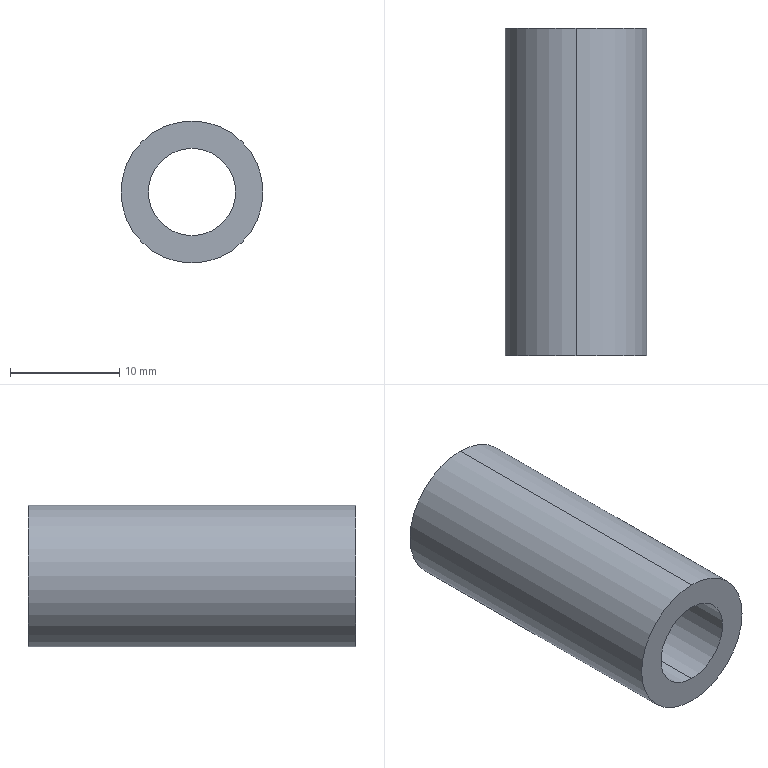Part | STEP file | Ball joint spacer | 1 solid | 6 faces | box 13 x 30 x 13 mm | volume 2474 mm3 | cylinder 4 | plane 2 | commonest cylinder face diameters 8 x2 13 x2
STEP:
#1=CARTESIAN_POINT('',(0.,0.,0.));
#2=DIRECTION('',(0.,0.,1.));
#3=DIRECTION('',(1.,0.,0.));
#4=AXIS2_PLACEMENT_3D('',#1,#2,#3);
#5=CARTESIAN_POINT('',(0.,30.,-4.));
#6=VERTEX_POINT('',#5);
#7=CARTESIAN_POINT('',(0.,0.,-4.));
#8=VERTEX_POINT('',#7);
#9=CARTESIAN_POINT('',(0.,30.,-4.));
#10=DIRECTION('',(0.,-1.,0.));
#11=VECTOR('',#10,1.);
#12=LINE('',#9,#11);
#13=CARTESIAN_POINT('',(0.,30.,0.));
#14=DIRECTION('',(0.,-1.,0.));
#15=DIRECTION('',(0.,0.,-1.));
#16=AXIS2_PLACEMENT_3D('',#13,#14,#15);
#17=CYLINDRICAL_SURFACE('',#16,4.);
#18=CARTESIAN_POINT('',(6.283,0.));
#19=DIRECTION('',(0.,1.));
#20=VECTOR('',#19,1.);
#21=LINE('',#18,#20);
#22=(GEOMETRIC_REPRESENTATION_CONTEXT(2)PARAMETRIC_REPRESENTATION_CONTEXT()REPRESENTATION_CONTEXT('',''));
#23=DEFINITIONAL_REPRESENTATION('',(#21),#22);
#24=PCURVE('',#17,#23);
#25=CARTESIAN_POINT('',(0.,30.,0.));
#26=DIRECTION('',(0.,-1.,0.));
#27=DIRECTION('',(0.,0.,-1.));
#28=AXIS2_PLACEMENT_3D('',#25,#26,#27);
#29=CYLINDRICAL_SURFACE('',#28,4.);
#30=CARTESIAN_POINT('',(0.,0.));
#31=DIRECTION('',(0.,1.));
#32=VECTOR('',#31,1.);
#33=LINE('',#30,#32);
#34=(GEOMETRIC_REPRESENTATION_CONTEXT(2)PARAMETRIC_REPRESENTATION_CONTEXT()REPRESENTATION_CONTEXT('',''));
#35=DEFINITIONAL_REPRESENTATION('',(#33),#34);
#36=PCURVE('',#29,#35);
#37=SURFACE_CURVE('',#12,(#24,#36),.PCURVE_S1.);
#38=EDGE_CURVE('',#6,#8,#37,.T.);
#39=ORIENTED_EDGE('',*,*,#38,.T.);
#40=CARTESIAN_POINT('',(0.,0.,4.));
#41=VERTEX_POINT('',#40);
#42=CARTESIAN_POINT('',(0.,0.,0.));
#43=DIRECTION('',(0.,1.,0.));
#44=DIRECTION('',(0.,0.,1.));
#45=AXIS2_PLACEMENT_3D('',#42,#43,#44);
#46=CIRCLE('',#45,4.);
#47=CARTESIAN_POINT('',(9.425,30.));
#48=DIRECTION('',(-1.,0.));
#49=VECTOR('',#48,1.);
#50=LINE('',#47,#49);
#51=(GEOMETRIC_REPRESENTATION_CONTEXT(2)PARAMETRIC_REPRESENTATION_CONTEXT()REPRESENTATION_CONTEXT('',''));
#52=DEFINITIONAL_REPRESENTATION('',(#50),#51);
#53=PCURVE('',#17,#52);
#54=CARTESIAN_POINT('',(0.,0.,0.));
#55=DIRECTION('',(0.,1.,0.));
#56=DIRECTION('',(0.,0.,1.));
#57=AXIS2_PLACEMENT_3D('',#54,#55,#56);
#58=PLANE('',#57);
#59=CARTESIAN_POINT('',(0.,0.));
#60=DIRECTION('',(1.,0.));
#61=AXIS2_PLACEMENT_2D('',#59,#60);
#62=CIRCLE('',#61,4.);
#63=(GEOMETRIC_REPRESENTATION_CONTEXT(2)PARAMETRIC_REPRESENTATION_CONTEXT()REPRESENTATION_CONTEXT('',''));
#64=DEFINITIONAL_REPRESENTATION('',(#62),#63);
#65=PCURVE('',#58,#64);
#66=SURFACE_CURVE('',#46,(#53,#65),.PCURVE_S1.);
#67=EDGE_CURVE('',#8,#41,#66,.T.);
#68=ORIENTED_EDGE('',*,*,#67,.T.);
#69=CARTESIAN_POINT('',(0.,30.,4.));
#70=VERTEX_POINT('',#69);
#71=CARTESIAN_POINT('',(0.,30.,4.));
#72=DIRECTION('',(0.,-1.,0.));
#73=VECTOR('',#72,1.);
#74=LINE('',#71,#73);
#75=CARTESIAN_POINT('',(3.142,0.));
#76=DIRECTION('',(0.,1.));
#77=VECTOR('',#76,1.);
#78=LINE('',#75,#77);
#79=(GEOMETRIC_REPRESENTATION_CONTEXT(2)PARAMETRIC_REPRESENTATION_CONTEXT()REPRESENTATION_CONTEXT('',''));
#80=DEFINITIONAL_REPRESENTATION('',(#78),#79);
#81=PCURVE('',#17,#80);
#82=CARTESIAN_POINT('',(3.142,0.));
#83=DIRECTION('',(0.,1.));
#84=VECTOR('',#83,1.);
#85=LINE('',#82,#84);
#86=(GEOMETRIC_REPRESENTATION_CONTEXT(2)PARAMETRIC_REPRESENTATION_CONTEXT()REPRESENTATION_CONTEXT('',''));
#87=DEFINITIONAL_REPRESENTATION('',(#85),#86);
#88=PCURVE('',#29,#87);
#89=SURFACE_CURVE('',#74,(#81,#88),.PCURVE_S1.);
#90=EDGE_CURVE('',#70,#41,#89,.T.);
#91=ORIENTED_EDGE('',*,*,#90,.F.);
#92=CARTESIAN_POINT('',(0.,30.,0.));
#93=DIRECTION('',(0.,1.,0.));
#94=DIRECTION('',(0.,0.,1.));
#95=AXIS2_PLACEMENT_3D('',#92,#93,#94);
#96=CIRCLE('',#95,4.);
#97=CARTESIAN_POINT('',(9.425,0.));
#98=DIRECTION('',(-1.,0.));
#99=VECTOR('',#98,1.);
#100=LINE('',#97,#99);
#101=(GEOMETRIC_REPRESENTATION_CONTEXT(2)PARAMETRIC_REPRESENTATION_CONTEXT()REPRESENTATION_CONTEXT('',''));
#102=DEFINITIONAL_REPRESENTATION('',(#100),#101);
#103=PCURVE('',#17,#102);
#104=CARTESIAN_POINT('',(0.,30.,0.));
#105=DIRECTION('',(0.,1.,0.));
#106=DIRECTION('',(0.,0.,1.));
#107=AXIS2_PLACEMENT_3D('',#104,#105,#106);
#108=PLANE('',#107);
#109=CARTESIAN_POINT('',(0.,0.));
#110=DIRECTION('',(1.,0.));
#111=AXIS2_PLACEMENT_2D('',#109,#110);
#112=CIRCLE('',#111,4.);
#113=(GEOMETRIC_REPRESENTATION_CONTEXT(2)PARAMETRIC_REPRESENTATION_CONTEXT()REPRESENTATION_CONTEXT('',''));
#114=DEFINITIONAL_REPRESENTATION('',(#112),#113);
#115=PCURVE('',#108,#114);
#116=SURFACE_CURVE('',#96,(#103,#115),.PCURVE_S1.);
#117=EDGE_CURVE('',#6,#70,#116,.T.);
#118=ORIENTED_EDGE('',*,*,#117,.F.);
#119=EDGE_LOOP('',(#39,#68,#91,#118));
#120=FACE_BOUND('',#119,.F.);
#121=ADVANCED_FACE('',(#120),#17,.F.);
#122=CARTESIAN_POINT('',(0.,30.,6.5));
#123=VERTEX_POINT('',#122);
#124=CARTESIAN_POINT('',(0.,30.,-6.5));
#125=VERTEX_POINT('',#124);
#126=CARTESIAN_POINT('',(0.,30.,0.));
#127=DIRECTION('',(0.,1.,0.));
#128=DIRECTION('',(0.,0.,1.));
#129=AXIS2_PLACEMENT_3D('',#126,#127,#128);
#130=CIRCLE('',#129,6.5);
#131=CARTESIAN_POINT('',(0.,30.,0.));
#132=DIRECTION('',(0.,-1.,0.));
#133=DIRECTION('',(0.,0.,-1.));
#134=AXIS2_PLACEMENT_3D('',#131,#132,#133);
#135=CYLINDRICAL_SURFACE('',#134,6.5);
#136=CARTESIAN_POINT('',(3.142,0.));
#137=DIRECTION('',(-1.,0.));
#138=VECTOR('',#137,1.);
#139=LINE('',#136,#138);
#140=(GEOMETRIC_REPRESENTATION_CONTEXT(2)PARAMETRIC_REPRESENTATION_CONTEXT()REPRESENTATION_CONTEXT('',''));
#141=DEFINITIONAL_REPRESENTATION('',(#139),#140);
#142=PCURVE('',#135,#141);
#143=CARTESIAN_POINT('',(0.,0.));
#144=DIRECTION('',(1.,0.));
#145=AXIS2_PLACEMENT_2D('',#143,#144);
#146=CIRCLE('',#145,6.5);
#147=(GEOMETRIC_REPRESENTATION_CONTEXT(2)PARAMETRIC_REPRESENTATION_CONTEXT()REPRESENTATION_CONTEXT('',''));
#148=DEFINITIONAL_REPRESENTATION('',(#146),#147);
#149=PCURVE('',#108,#148);
#150=SURFACE_CURVE('',#130,(#142,#149),.PCURVE_S1.);
#151=EDGE_CURVE('',#123,#125,#150,.T.);
#152=ORIENTED_EDGE('',*,*,#151,.F.);
#153=CARTESIAN_POINT('',(0.,0.,6.5));
#154=VERTEX_POINT('',#153);
#155=CARTESIAN_POINT('',(0.,30.,6.5));
#156=DIRECTION('',(0.,-1.,0.));
#157=VECTOR('',#156,1.);
#158=LINE('',#155,#157);
#159=CARTESIAN_POINT('',(3.142,0.));
#160=DIRECTION('',(0.,1.));
#161=VECTOR('',#160,1.);
#162=LINE('',#159,#161);
#163=(GEOMETRIC_REPRESENTATION_CONTEXT(2)PARAMETRIC_REPRESENTATION_CONTEXT()REPRESENTATION_CONTEXT('',''));
#164=DEFINITIONAL_REPRESENTATION('',(#162),#163);
#165=PCURVE('',#135,#164);
#166=CARTESIAN_POINT('',(0.,30.,0.));
#167=DIRECTION('',(0.,-1.,0.));
#168=DIRECTION('',(0.,0.,-1.));
#169=AXIS2_PLACEMENT_3D('',#166,#167,#168);
#170=CYLINDRICAL_SURFACE('',#169,6.5);
#171=CARTESIAN_POINT('',(3.142,0.));
#172=DIRECTION('',(0.,1.));
#173=VECTOR('',#172,1.);
#174=LINE('',#171,#173);
#175=(GEOMETRIC_REPRESENTATION_CONTEXT(2)PARAMETRIC_REPRESENTATION_CONTEXT()REPRESENTATION_CONTEXT('',''));
#176=DEFINITIONAL_REPRESENTATION('',(#174),#175);
#177=PCURVE('',#170,#176);
#178=SURFACE_CURVE('',#158,(#165,#177),.PCURVE_S1.);
#179=EDGE_CURVE('',#123,#154,#178,.T.);
#180=ORIENTED_EDGE('',*,*,#179,.T.);
#181=CARTESIAN_POINT('',(0.,0.,-6.5));
#182=VERTEX_POINT('',#181);
#183=CARTESIAN_POINT('',(0.,0.,0.));
#184=DIRECTION('',(0.,1.,0.));
#185=DIRECTION('',(0.,0.,1.));
#186=AXIS2_PLACEMENT_3D('',#183,#184,#185);
#187=CIRCLE('',#186,6.5);
#188=CARTESIAN_POINT('',(3.142,30.));
#189=DIRECTION('',(-1.,0.));
#190=VECTOR('',#189,1.);
#191=LINE('',#188,#190);
#192=(GEOMETRIC_REPRESENTATION_CONTEXT(2)PARAMETRIC_REPRESENTATION_CONTEXT()REPRESENTATION_CONTEXT('',''));
#193=DEFINITIONAL_REPRESENTATION('',(#191),#192);
#194=PCURVE('',#135,#193);
#195=CARTESIAN_POINT('',(0.,0.));
#196=DIRECTION('',(1.,0.));
#197=AXIS2_PLACEMENT_2D('',#195,#196);
#198=CIRCLE('',#197,6.5);
#199=(GEOMETRIC_REPRESENTATION_CONTEXT(2)PARAMETRIC_REPRESENTATION_CONTEXT()REPRESENTATION_CONTEXT('',''));
#200=DEFINITIONAL_REPRESENTATION('',(#198),#199);
#201=PCURVE('',#58,#200);
#202=SURFACE_CURVE('',#187,(#194,#201),.PCURVE_S1.);
#203=EDGE_CURVE('',#154,#182,#202,.T.);
#204=ORIENTED_EDGE('',*,*,#203,.T.);
#205=CARTESIAN_POINT('',(0.,30.,-6.5));
#206=DIRECTION('',(0.,-1.,0.));
#207=VECTOR('',#206,1.);
#208=LINE('',#205,#207);
#209=CARTESIAN_POINT('',(0.,0.));
#210=DIRECTION('',(0.,1.));
#211=VECTOR('',#210,1.);
#212=LINE('',#209,#211);
#213=(GEOMETRIC_REPRESENTATION_CONTEXT(2)PARAMETRIC_REPRESENTATION_CONTEXT()REPRESENTATION_CONTEXT('',''));
#214=DEFINITIONAL_REPRESENTATION('',(#212),#213);
#215=PCURVE('',#135,#214);
#216=CARTESIAN_POINT('',(6.283,0.));
#217=DIRECTION('',(0.,1.));
#218=VECTOR('',#217,1.);
#219=LINE('',#216,#218);
#220=(GEOMETRIC_REPRESENTATION_CONTEXT(2)PARAMETRIC_REPRESENTATION_CONTEXT()REPRESENTATION_CONTEXT('',''));
#221=DEFINITIONAL_REPRESENTATION('',(#219),#220);
#222=PCURVE('',#170,#221);
#223=SURFACE_CURVE('',#208,(#215,#222),.PCURVE_S1.);
#224=EDGE_CURVE('',#125,#182,#223,.T.);
#225=ORIENTED_EDGE('',*,*,#224,.F.);
#226=EDGE_LOOP('',(#152,#180,#204,#225));
#227=FACE_BOUND('',#226,.T.);
#228=ADVANCED_FACE('',(#227),#135,.T.);
#229=CARTESIAN_POINT('',(0.,30.,0.));
#230=DIRECTION('',(0.,1.,0.));
#231=DIRECTION('',(0.,0.,1.));
#232=AXIS2_PLACEMENT_3D('',#229,#230,#231);
#233=CIRCLE('',#232,6.5);
#234=CARTESIAN_POINT('',(0.,0.));
#235=DIRECTION('',(1.,0.));
#236=AXIS2_PLACEMENT_2D('',#234,#235);
#237=CIRCLE('',#236,6.5);
#238=(GEOMETRIC_REPRESENTATION_CONTEXT(2)PARAMETRIC_REPRESENTATION_CONTEXT()REPRESENTATION_CONTEXT('',''));
#239=DEFINITIONAL_REPRESENTATION('',(#237),#238);
#240=PCURVE('',#108,#239);
#241=CARTESIAN_POINT('',(9.425,0.));
#242=DIRECTION('',(-1.,0.));
#243=VECTOR('',#242,1.);
#244=LINE('',#241,#243);
#245=(GEOMETRIC_REPRESENTATION_CONTEXT(2)PARAMETRIC_REPRESENTATION_CONTEXT()REPRESENTATION_CONTEXT('',''));
#246=DEFINITIONAL_REPRESENTATION('',(#244),#245);
#247=PCURVE('',#170,#246);
#248=SURFACE_CURVE('',#233,(#240,#247),.PCURVE_S1.);
#249=EDGE_CURVE('',#125,#123,#248,.T.);
#250=ORIENTED_EDGE('',*,*,#249,.T.);
#251=ORIENTED_EDGE('',*,*,#151,.T.);
#252=EDGE_LOOP('',(#250,#251));
#253=FACE_BOUND('',#252,.T.);
#254=ORIENTED_EDGE('',*,*,#117,.F.);
#255=CARTESIAN_POINT('',(0.,30.,0.));
#256=DIRECTION('',(0.,1.,0.));
#257=DIRECTION('',(0.,0.,1.));
#258=AXIS2_PLACEMENT_3D('',#255,#256,#257);
#259=CIRCLE('',#258,4.);
#260=CARTESIAN_POINT('',(0.,0.));
#261=DIRECTION('',(1.,0.));
#262=AXIS2_PLACEMENT_2D('',#260,#261);
#263=CIRCLE('',#262,4.);
#264=(GEOMETRIC_REPRESENTATION_CONTEXT(2)PARAMETRIC_REPRESENTATION_CONTEXT()REPRESENTATION_CONTEXT('',''));
#265=DEFINITIONAL_REPRESENTATION('',(#263),#264);
#266=PCURVE('',#108,#265);
#267=CARTESIAN_POINT('',(3.142,0.));
#268=DIRECTION('',(-1.,0.));
#269=VECTOR('',#268,1.);
#270=LINE('',#267,#269);
#271=(GEOMETRIC_REPRESENTATION_CONTEXT(2)PARAMETRIC_REPRESENTATION_CONTEXT()REPRESENTATION_CONTEXT('',''));
#272=DEFINITIONAL_REPRESENTATION('',(#270),#271);
#273=PCURVE('',#29,#272);
#274=SURFACE_CURVE('',#259,(#266,#273),.PCURVE_S1.);
#275=EDGE_CURVE('',#70,#6,#274,.T.);
#276=ORIENTED_EDGE('',*,*,#275,.F.);
#277=EDGE_LOOP('',(#254,#276));
#278=FACE_BOUND('',#277,.T.);
#279=ADVANCED_FACE('',(#253,#278),#108,.T.);
#280=CARTESIAN_POINT('',(0.,0.,0.));
#281=DIRECTION('',(0.,1.,0.));
#282=DIRECTION('',(0.,0.,1.));
#283=AXIS2_PLACEMENT_3D('',#280,#281,#282);
#284=CIRCLE('',#283,6.5);
#285=CARTESIAN_POINT('',(0.,0.));
#286=DIRECTION('',(1.,0.));
#287=AXIS2_PLACEMENT_2D('',#285,#286);
#288=CIRCLE('',#287,6.5);
#289=(GEOMETRIC_REPRESENTATION_CONTEXT(2)PARAMETRIC_REPRESENTATION_CONTEXT()REPRESENTATION_CONTEXT('',''));
#290=DEFINITIONAL_REPRESENTATION('',(#288),#289);
#291=PCURVE('',#58,#290);
#292=CARTESIAN_POINT('',(9.425,30.));
#293=DIRECTION('',(-1.,0.));
#294=VECTOR('',#293,1.);
#295=LINE('',#292,#294);
#296=(GEOMETRIC_REPRESENTATION_CONTEXT(2)PARAMETRIC_REPRESENTATION_CONTEXT()REPRESENTATION_CONTEXT('',''));
#297=DEFINITIONAL_REPRESENTATION('',(#295),#296);
#298=PCURVE('',#170,#297);
#299=SURFACE_CURVE('',#284,(#291,#298),.PCURVE_S1.);
#300=EDGE_CURVE('',#182,#154,#299,.T.);
#301=ORIENTED_EDGE('',*,*,#300,.F.);
#302=ORIENTED_EDGE('',*,*,#203,.F.);
#303=EDGE_LOOP('',(#301,#302));
#304=FACE_BOUND('',#303,.T.);
#305=ORIENTED_EDGE('',*,*,#67,.T.);
#306=CARTESIAN_POINT('',(0.,0.,0.));
#307=DIRECTION('',(0.,1.,0.));
#308=DIRECTION('',(0.,0.,1.));
#309=AXIS2_PLACEMENT_3D('',#306,#307,#308);
#310=CIRCLE('',#309,4.);
#311=CARTESIAN_POINT('',(0.,0.));
#312=DIRECTION('',(1.,0.));
#313=AXIS2_PLACEMENT_2D('',#311,#312);
#314=CIRCLE('',#313,4.);
#315=(GEOMETRIC_REPRESENTATION_CONTEXT(2)PARAMETRIC_REPRESENTATION_CONTEXT()REPRESENTATION_CONTEXT('',''));
#316=DEFINITIONAL_REPRESENTATION('',(#314),#315);
#317=PCURVE('',#58,#316);
#318=CARTESIAN_POINT('',(3.142,30.));
#319=DIRECTION('',(-1.,0.));
#320=VECTOR('',#319,1.);
#321=LINE('',#318,#320);
#322=(GEOMETRIC_REPRESENTATION_CONTEXT(2)PARAMETRIC_REPRESENTATION_CONTEXT()REPRESENTATION_CONTEXT('',''));
#323=DEFINITIONAL_REPRESENTATION('',(#321),#322);
#324=PCURVE('',#29,#323);
#325=SURFACE_CURVE('',#310,(#317,#324),.PCURVE_S1.);
#326=EDGE_CURVE('',#41,#8,#325,.T.);
#327=ORIENTED_EDGE('',*,*,#326,.T.);
#328=EDGE_LOOP('',(#305,#327));
#329=FACE_BOUND('',#328,.T.);
#330=ADVANCED_FACE('',(#304,#329),#58,.F.);
#331=ORIENTED_EDGE('',*,*,#179,.F.);
#332=ORIENTED_EDGE('',*,*,#249,.F.);
#333=ORIENTED_EDGE('',*,*,#224,.T.);
#334=ORIENTED_EDGE('',*,*,#300,.T.);
#335=EDGE_LOOP('',(#331,#332,#333,#334));
#336=FACE_BOUND('',#335,.T.);
#337=ADVANCED_FACE('',(#336),#170,.T.);
#338=ORIENTED_EDGE('',*,*,#326,.T.);
#339=ORIENTED_EDGE('',*,*,#38,.F.);
#340=ORIENTED_EDGE('',*,*,#275,.F.);
#341=ORIENTED_EDGE('',*,*,#90,.T.);
#342=EDGE_LOOP('',(#338,#339,#340,#341));
#343=FACE_BOUND('',#342,.F.);
#344=ADVANCED_FACE('',(#343),#29,.F.);
#345=CLOSED_SHELL('',(#121,#228,#279,#330,#337,#344));
#346=MANIFOLD_SOLID_BREP('',#345);
#347=(LENGTH_UNIT()NAMED_UNIT(*)SI_UNIT(.MILLI.,.METRE.));
#348=UNCERTAINTY_MEASURE_WITH_UNIT(LENGTH_MEASURE(0.0000001),#347,'','');
#349=(NAMED_UNIT(*)PLANE_ANGLE_UNIT()SI_UNIT($,.RADIAN.));
#350=(NAMED_UNIT(*)SI_UNIT($,.STERADIAN.)SOLID_ANGLE_UNIT());
#351=(GEOMETRIC_REPRESENTATION_CONTEXT(3)GLOBAL_UNCERTAINTY_ASSIGNED_CONTEXT((#348))GLOBAL_UNIT_ASSIGNED_CONTEXT((#347,#349,#350))REPRESENTATION_CONTEXT('',''));
#352=ADVANCED_BREP_SHAPE_REPRESENTATION('',(#4,#346),#351);